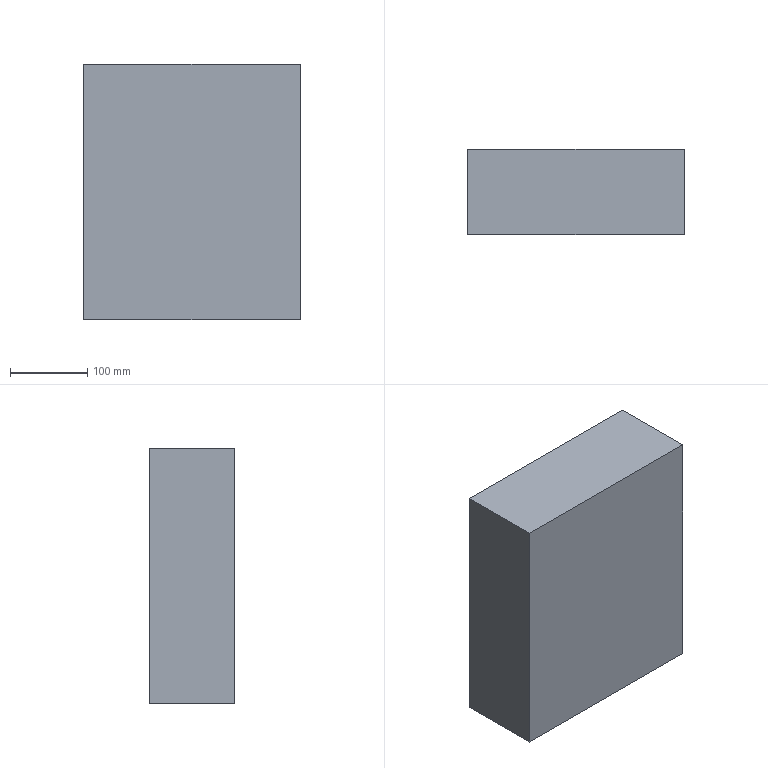Part | STEP file | 0230_Work-A | 1 solid | 6 faces | box 280 x 110 x 330 mm | volume 10164000 mm3 | plane 6
STEP:
#1=CARTESIAN_POINT('',(0.,0.,0.));
#2=DIRECTION('',(0.,0.,1.));
#3=DIRECTION('',(1.,0.,0.));
#4=AXIS2_PLACEMENT_3D('',#1,#2,#3);
#5=CARTESIAN_POINT('',(-140.,0.,-330.));
#6=VERTEX_POINT('',#5);
#7=CARTESIAN_POINT('',(-140.,0.,0.));
#8=VERTEX_POINT('',#7);
#9=CARTESIAN_POINT('',(-140.,0.,0.));
#10=DIRECTION('',(0.,0.,1.));
#11=VECTOR('',#10,1.);
#12=LINE('',#9,#11);
#13=CARTESIAN_POINT('',(-140.,110.,0.));
#14=DIRECTION('',(1.,0.,0.));
#15=DIRECTION('',(0.,0.,-1.));
#16=AXIS2_PLACEMENT_3D('',#13,#14,#15);
#17=PLANE('',#16);
#18=CARTESIAN_POINT('',(0.,-110.));
#19=DIRECTION('',(-1.,0.));
#20=VECTOR('',#19,1.);
#21=LINE('',#18,#20);
#22=(GEOMETRIC_REPRESENTATION_CONTEXT(2)PARAMETRIC_REPRESENTATION_CONTEXT()REPRESENTATION_CONTEXT('',''));
#23=DEFINITIONAL_REPRESENTATION('',(#21),#22);
#24=PCURVE('',#17,#23);
#25=CARTESIAN_POINT('',(-140.,0.,-330.));
#26=DIRECTION('',(0.,-1.,0.));
#27=DIRECTION('',(0.,0.,-1.));
#28=AXIS2_PLACEMENT_3D('',#25,#26,#27);
#29=PLANE('',#28);
#30=CARTESIAN_POINT('',(-330.,0.));
#31=DIRECTION('',(-1.,0.));
#32=VECTOR('',#31,1.);
#33=LINE('',#30,#32);
#34=(GEOMETRIC_REPRESENTATION_CONTEXT(2)PARAMETRIC_REPRESENTATION_CONTEXT()REPRESENTATION_CONTEXT('',''));
#35=DEFINITIONAL_REPRESENTATION('',(#33),#34);
#36=PCURVE('',#29,#35);
#37=SURFACE_CURVE('',#12,(#24,#36),.PCURVE_S1.);
#38=EDGE_CURVE('',#6,#8,#37,.T.);
#39=ORIENTED_EDGE('',*,*,#38,.T.);
#40=CARTESIAN_POINT('',(-140.,110.,0.));
#41=VERTEX_POINT('',#40);
#42=CARTESIAN_POINT('',(-140.,110.,0.));
#43=DIRECTION('',(0.,-1.,0.));
#44=VECTOR('',#43,1.);
#45=LINE('',#42,#44);
#46=CARTESIAN_POINT('',(0.,0.));
#47=DIRECTION('',(0.,-1.));
#48=VECTOR('',#47,1.);
#49=LINE('',#46,#48);
#50=(GEOMETRIC_REPRESENTATION_CONTEXT(2)PARAMETRIC_REPRESENTATION_CONTEXT()REPRESENTATION_CONTEXT('',''));
#51=DEFINITIONAL_REPRESENTATION('',(#49),#50);
#52=PCURVE('',#17,#51);
#53=CARTESIAN_POINT('',(-140.,110.,0.));
#54=DIRECTION('',(0.,0.,-1.));
#55=DIRECTION('',(-1.,0.,0.));
#56=AXIS2_PLACEMENT_3D('',#53,#54,#55);
#57=PLANE('',#56);
#58=CARTESIAN_POINT('',(0.,0.));
#59=DIRECTION('',(0.,-1.));
#60=VECTOR('',#59,1.);
#61=LINE('',#58,#60);
#62=(GEOMETRIC_REPRESENTATION_CONTEXT(2)PARAMETRIC_REPRESENTATION_CONTEXT()REPRESENTATION_CONTEXT('',''));
#63=DEFINITIONAL_REPRESENTATION('',(#61),#62);
#64=PCURVE('',#57,#63);
#65=SURFACE_CURVE('',#45,(#52,#64),.PCURVE_S1.);
#66=EDGE_CURVE('',#41,#8,#65,.T.);
#67=ORIENTED_EDGE('',*,*,#66,.F.);
#68=CARTESIAN_POINT('',(-140.,110.,-330.));
#69=VERTEX_POINT('',#68);
#70=CARTESIAN_POINT('',(-140.,110.,0.));
#71=DIRECTION('',(0.,0.,1.));
#72=VECTOR('',#71,1.);
#73=LINE('',#70,#72);
#74=CARTESIAN_POINT('',(0.,0.));
#75=DIRECTION('',(-1.,0.));
#76=VECTOR('',#75,1.);
#77=LINE('',#74,#76);
#78=(GEOMETRIC_REPRESENTATION_CONTEXT(2)PARAMETRIC_REPRESENTATION_CONTEXT()REPRESENTATION_CONTEXT('',''));
#79=DEFINITIONAL_REPRESENTATION('',(#77),#78);
#80=PCURVE('',#17,#79);
#81=CARTESIAN_POINT('',(-140.,110.,-330.));
#82=DIRECTION('',(0.,-1.,0.));
#83=DIRECTION('',(0.,0.,-1.));
#84=AXIS2_PLACEMENT_3D('',#81,#82,#83);
#85=PLANE('',#84);
#86=CARTESIAN_POINT('',(-330.,0.));
#87=DIRECTION('',(-1.,0.));
#88=VECTOR('',#87,1.);
#89=LINE('',#86,#88);
#90=(GEOMETRIC_REPRESENTATION_CONTEXT(2)PARAMETRIC_REPRESENTATION_CONTEXT()REPRESENTATION_CONTEXT('',''));
#91=DEFINITIONAL_REPRESENTATION('',(#89),#90);
#92=PCURVE('',#85,#91);
#93=SURFACE_CURVE('',#73,(#80,#92),.PCURVE_S1.);
#94=EDGE_CURVE('',#69,#41,#93,.T.);
#95=ORIENTED_EDGE('',*,*,#94,.F.);
#96=CARTESIAN_POINT('',(-140.,110.,-330.));
#97=DIRECTION('',(0.,-1.,0.));
#98=VECTOR('',#97,1.);
#99=LINE('',#96,#98);
#100=CARTESIAN_POINT('',(330.,0.));
#101=DIRECTION('',(0.,-1.));
#102=VECTOR('',#101,1.);
#103=LINE('',#100,#102);
#104=(GEOMETRIC_REPRESENTATION_CONTEXT(2)PARAMETRIC_REPRESENTATION_CONTEXT()REPRESENTATION_CONTEXT('',''));
#105=DEFINITIONAL_REPRESENTATION('',(#103),#104);
#106=PCURVE('',#17,#105);
#107=CARTESIAN_POINT('',(-140.,110.,-330.));
#108=DIRECTION('',(0.,0.,1.));
#109=DIRECTION('',(1.,0.,0.));
#110=AXIS2_PLACEMENT_3D('',#107,#108,#109);
#111=PLANE('',#110);
#112=CARTESIAN_POINT('',(0.,0.));
#113=DIRECTION('',(0.,-1.));
#114=VECTOR('',#113,1.);
#115=LINE('',#112,#114);
#116=(GEOMETRIC_REPRESENTATION_CONTEXT(2)PARAMETRIC_REPRESENTATION_CONTEXT()REPRESENTATION_CONTEXT('',''));
#117=DEFINITIONAL_REPRESENTATION('',(#115),#116);
#118=PCURVE('',#111,#117);
#119=SURFACE_CURVE('',#99,(#106,#118),.PCURVE_S1.);
#120=EDGE_CURVE('',#69,#6,#119,.T.);
#121=ORIENTED_EDGE('',*,*,#120,.T.);
#122=EDGE_LOOP('',(#39,#67,#95,#121));
#123=FACE_BOUND('',#122,.T.);
#124=ADVANCED_FACE('',(#123),#17,.F.);
#125=CARTESIAN_POINT('',(140.,0.,0.));
#126=VERTEX_POINT('',#125);
#127=CARTESIAN_POINT('',(-140.,0.,0.));
#128=DIRECTION('',(1.,0.,0.));
#129=VECTOR('',#128,1.);
#130=LINE('',#127,#129);
#131=CARTESIAN_POINT('',(0.,-110.));
#132=DIRECTION('',(-1.,0.));
#133=VECTOR('',#132,1.);
#134=LINE('',#131,#133);
#135=(GEOMETRIC_REPRESENTATION_CONTEXT(2)PARAMETRIC_REPRESENTATION_CONTEXT()REPRESENTATION_CONTEXT('',''));
#136=DEFINITIONAL_REPRESENTATION('',(#134),#135);
#137=PCURVE('',#57,#136);
#138=CARTESIAN_POINT('',(-330.,0.));
#139=DIRECTION('',(0.,1.));
#140=VECTOR('',#139,1.);
#141=LINE('',#138,#140);
#142=(GEOMETRIC_REPRESENTATION_CONTEXT(2)PARAMETRIC_REPRESENTATION_CONTEXT()REPRESENTATION_CONTEXT('',''));
#143=DEFINITIONAL_REPRESENTATION('',(#141),#142);
#144=PCURVE('',#29,#143);
#145=SURFACE_CURVE('',#130,(#137,#144),.PCURVE_S1.);
#146=EDGE_CURVE('',#8,#126,#145,.T.);
#147=ORIENTED_EDGE('',*,*,#146,.T.);
#148=CARTESIAN_POINT('',(140.,110.,0.));
#149=VERTEX_POINT('',#148);
#150=CARTESIAN_POINT('',(140.,110.,0.));
#151=DIRECTION('',(0.,-1.,0.));
#152=VECTOR('',#151,1.);
#153=LINE('',#150,#152);
#154=CARTESIAN_POINT('',(-280.,0.));
#155=DIRECTION('',(0.,-1.));
#156=VECTOR('',#155,1.);
#157=LINE('',#154,#156);
#158=(GEOMETRIC_REPRESENTATION_CONTEXT(2)PARAMETRIC_REPRESENTATION_CONTEXT()REPRESENTATION_CONTEXT('',''));
#159=DEFINITIONAL_REPRESENTATION('',(#157),#158);
#160=PCURVE('',#57,#159);
#161=CARTESIAN_POINT('',(140.,110.,0.));
#162=DIRECTION('',(-1.,0.,0.));
#163=DIRECTION('',(0.,0.,1.));
#164=AXIS2_PLACEMENT_3D('',#161,#162,#163);
#165=PLANE('',#164);
#166=CARTESIAN_POINT('',(0.,0.));
#167=DIRECTION('',(0.,-1.));
#168=VECTOR('',#167,1.);
#169=LINE('',#166,#168);
#170=(GEOMETRIC_REPRESENTATION_CONTEXT(2)PARAMETRIC_REPRESENTATION_CONTEXT()REPRESENTATION_CONTEXT('',''));
#171=DEFINITIONAL_REPRESENTATION('',(#169),#170);
#172=PCURVE('',#165,#171);
#173=SURFACE_CURVE('',#153,(#160,#172),.PCURVE_S1.);
#174=EDGE_CURVE('',#149,#126,#173,.T.);
#175=ORIENTED_EDGE('',*,*,#174,.F.);
#176=CARTESIAN_POINT('',(-140.,110.,0.));
#177=DIRECTION('',(1.,0.,0.));
#178=VECTOR('',#177,1.);
#179=LINE('',#176,#178);
#180=CARTESIAN_POINT('',(0.,0.));
#181=DIRECTION('',(-1.,0.));
#182=VECTOR('',#181,1.);
#183=LINE('',#180,#182);
#184=(GEOMETRIC_REPRESENTATION_CONTEXT(2)PARAMETRIC_REPRESENTATION_CONTEXT()REPRESENTATION_CONTEXT('',''));
#185=DEFINITIONAL_REPRESENTATION('',(#183),#184);
#186=PCURVE('',#57,#185);
#187=CARTESIAN_POINT('',(-330.,0.));
#188=DIRECTION('',(0.,1.));
#189=VECTOR('',#188,1.);
#190=LINE('',#187,#189);
#191=(GEOMETRIC_REPRESENTATION_CONTEXT(2)PARAMETRIC_REPRESENTATION_CONTEXT()REPRESENTATION_CONTEXT('',''));
#192=DEFINITIONAL_REPRESENTATION('',(#190),#191);
#193=PCURVE('',#85,#192);
#194=SURFACE_CURVE('',#179,(#186,#193),.PCURVE_S1.);
#195=EDGE_CURVE('',#41,#149,#194,.T.);
#196=ORIENTED_EDGE('',*,*,#195,.F.);
#197=ORIENTED_EDGE('',*,*,#66,.T.);
#198=EDGE_LOOP('',(#147,#175,#196,#197));
#199=FACE_BOUND('',#198,.T.);
#200=ADVANCED_FACE('',(#199),#57,.F.);
#201=CARTESIAN_POINT('',(140.,0.,-330.));
#202=VERTEX_POINT('',#201);
#203=CARTESIAN_POINT('',(140.,0.,0.));
#204=DIRECTION('',(0.,0.,-1.));
#205=VECTOR('',#204,1.);
#206=LINE('',#203,#205);
#207=CARTESIAN_POINT('',(0.,-110.));
#208=DIRECTION('',(-1.,0.));
#209=VECTOR('',#208,1.);
#210=LINE('',#207,#209);
#211=(GEOMETRIC_REPRESENTATION_CONTEXT(2)PARAMETRIC_REPRESENTATION_CONTEXT()REPRESENTATION_CONTEXT('',''));
#212=DEFINITIONAL_REPRESENTATION('',(#210),#211);
#213=PCURVE('',#165,#212);
#214=CARTESIAN_POINT('',(-330.,280.));
#215=DIRECTION('',(1.,0.));
#216=VECTOR('',#215,1.);
#217=LINE('',#214,#216);
#218=(GEOMETRIC_REPRESENTATION_CONTEXT(2)PARAMETRIC_REPRESENTATION_CONTEXT()REPRESENTATION_CONTEXT('',''));
#219=DEFINITIONAL_REPRESENTATION('',(#217),#218);
#220=PCURVE('',#29,#219);
#221=SURFACE_CURVE('',#206,(#213,#220),.PCURVE_S1.);
#222=EDGE_CURVE('',#126,#202,#221,.T.);
#223=ORIENTED_EDGE('',*,*,#222,.T.);
#224=CARTESIAN_POINT('',(140.,110.,-330.));
#225=VERTEX_POINT('',#224);
#226=CARTESIAN_POINT('',(140.,110.,-330.));
#227=DIRECTION('',(0.,-1.,0.));
#228=VECTOR('',#227,1.);
#229=LINE('',#226,#228);
#230=CARTESIAN_POINT('',(-330.,0.));
#231=DIRECTION('',(0.,-1.));
#232=VECTOR('',#231,1.);
#233=LINE('',#230,#232);
#234=(GEOMETRIC_REPRESENTATION_CONTEXT(2)PARAMETRIC_REPRESENTATION_CONTEXT()REPRESENTATION_CONTEXT('',''));
#235=DEFINITIONAL_REPRESENTATION('',(#233),#234);
#236=PCURVE('',#165,#235);
#237=CARTESIAN_POINT('',(280.,0.));
#238=DIRECTION('',(0.,-1.));
#239=VECTOR('',#238,1.);
#240=LINE('',#237,#239);
#241=(GEOMETRIC_REPRESENTATION_CONTEXT(2)PARAMETRIC_REPRESENTATION_CONTEXT()REPRESENTATION_CONTEXT('',''));
#242=DEFINITIONAL_REPRESENTATION('',(#240),#241);
#243=PCURVE('',#111,#242);
#244=SURFACE_CURVE('',#229,(#236,#243),.PCURVE_S1.);
#245=EDGE_CURVE('',#225,#202,#244,.T.);
#246=ORIENTED_EDGE('',*,*,#245,.F.);
#247=CARTESIAN_POINT('',(140.,110.,0.));
#248=DIRECTION('',(0.,0.,-1.));
#249=VECTOR('',#248,1.);
#250=LINE('',#247,#249);
#251=CARTESIAN_POINT('',(0.,0.));
#252=DIRECTION('',(-1.,0.));
#253=VECTOR('',#252,1.);
#254=LINE('',#251,#253);
#255=(GEOMETRIC_REPRESENTATION_CONTEXT(2)PARAMETRIC_REPRESENTATION_CONTEXT()REPRESENTATION_CONTEXT('',''));
#256=DEFINITIONAL_REPRESENTATION('',(#254),#255);
#257=PCURVE('',#165,#256);
#258=CARTESIAN_POINT('',(-330.,280.));
#259=DIRECTION('',(1.,0.));
#260=VECTOR('',#259,1.);
#261=LINE('',#258,#260);
#262=(GEOMETRIC_REPRESENTATION_CONTEXT(2)PARAMETRIC_REPRESENTATION_CONTEXT()REPRESENTATION_CONTEXT('',''));
#263=DEFINITIONAL_REPRESENTATION('',(#261),#262);
#264=PCURVE('',#85,#263);
#265=SURFACE_CURVE('',#250,(#257,#264),.PCURVE_S1.);
#266=EDGE_CURVE('',#149,#225,#265,.T.);
#267=ORIENTED_EDGE('',*,*,#266,.F.);
#268=ORIENTED_EDGE('',*,*,#174,.T.);
#269=EDGE_LOOP('',(#223,#246,#267,#268));
#270=FACE_BOUND('',#269,.T.);
#271=ADVANCED_FACE('',(#270),#165,.F.);
#272=CARTESIAN_POINT('',(-140.,0.,-330.));
#273=DIRECTION('',(-1.,0.,0.));
#274=VECTOR('',#273,1.);
#275=LINE('',#272,#274);
#276=CARTESIAN_POINT('',(0.,-110.));
#277=DIRECTION('',(-1.,0.));
#278=VECTOR('',#277,1.);
#279=LINE('',#276,#278);
#280=(GEOMETRIC_REPRESENTATION_CONTEXT(2)PARAMETRIC_REPRESENTATION_CONTEXT()REPRESENTATION_CONTEXT('',''));
#281=DEFINITIONAL_REPRESENTATION('',(#279),#280);
#282=PCURVE('',#111,#281);
#283=CARTESIAN_POINT('',(0.,0.));
#284=DIRECTION('',(0.,-1.));
#285=VECTOR('',#284,1.);
#286=LINE('',#283,#285);
#287=(GEOMETRIC_REPRESENTATION_CONTEXT(2)PARAMETRIC_REPRESENTATION_CONTEXT()REPRESENTATION_CONTEXT('',''));
#288=DEFINITIONAL_REPRESENTATION('',(#286),#287);
#289=PCURVE('',#29,#288);
#290=SURFACE_CURVE('',#275,(#282,#289),.PCURVE_S1.);
#291=EDGE_CURVE('',#202,#6,#290,.T.);
#292=ORIENTED_EDGE('',*,*,#291,.T.);
#293=ORIENTED_EDGE('',*,*,#120,.F.);
#294=CARTESIAN_POINT('',(-140.,110.,-330.));
#295=DIRECTION('',(-1.,0.,0.));
#296=VECTOR('',#295,1.);
#297=LINE('',#294,#296);
#298=CARTESIAN_POINT('',(0.,0.));
#299=DIRECTION('',(-1.,0.));
#300=VECTOR('',#299,1.);
#301=LINE('',#298,#300);
#302=(GEOMETRIC_REPRESENTATION_CONTEXT(2)PARAMETRIC_REPRESENTATION_CONTEXT()REPRESENTATION_CONTEXT('',''));
#303=DEFINITIONAL_REPRESENTATION('',(#301),#302);
#304=PCURVE('',#111,#303);
#305=CARTESIAN_POINT('',(0.,0.));
#306=DIRECTION('',(0.,-1.));
#307=VECTOR('',#306,1.);
#308=LINE('',#305,#307);
#309=(GEOMETRIC_REPRESENTATION_CONTEXT(2)PARAMETRIC_REPRESENTATION_CONTEXT()REPRESENTATION_CONTEXT('',''));
#310=DEFINITIONAL_REPRESENTATION('',(#308),#309);
#311=PCURVE('',#85,#310);
#312=SURFACE_CURVE('',#297,(#304,#311),.PCURVE_S1.);
#313=EDGE_CURVE('',#225,#69,#312,.T.);
#314=ORIENTED_EDGE('',*,*,#313,.F.);
#315=ORIENTED_EDGE('',*,*,#245,.T.);
#316=EDGE_LOOP('',(#292,#293,#314,#315));
#317=FACE_BOUND('',#316,.T.);
#318=ADVANCED_FACE('',(#317),#111,.F.);
#319=ORIENTED_EDGE('',*,*,#94,.T.);
#320=ORIENTED_EDGE('',*,*,#195,.T.);
#321=ORIENTED_EDGE('',*,*,#266,.T.);
#322=ORIENTED_EDGE('',*,*,#313,.T.);
#323=EDGE_LOOP('',(#319,#320,#321,#322));
#324=FACE_BOUND('',#323,.T.);
#325=ADVANCED_FACE('',(#324),#85,.F.);
#326=ORIENTED_EDGE('',*,*,#38,.F.);
#327=ORIENTED_EDGE('',*,*,#291,.F.);
#328=ORIENTED_EDGE('',*,*,#222,.F.);
#329=ORIENTED_EDGE('',*,*,#146,.F.);
#330=EDGE_LOOP('',(#326,#327,#328,#329));
#331=FACE_BOUND('',#330,.T.);
#332=ADVANCED_FACE('',(#331),#29,.T.);
#333=CLOSED_SHELL('',(#124,#200,#271,#318,#325,#332));
#334=MANIFOLD_SOLID_BREP('',#333);
#335=(LENGTH_UNIT()NAMED_UNIT(*)SI_UNIT(.MILLI.,.METRE.));
#336=UNCERTAINTY_MEASURE_WITH_UNIT(LENGTH_MEASURE(0.0000001),#335,'','');
#337=(NAMED_UNIT(*)PLANE_ANGLE_UNIT()SI_UNIT($,.RADIAN.));
#338=(NAMED_UNIT(*)SI_UNIT($,.STERADIAN.)SOLID_ANGLE_UNIT());
#339=(GEOMETRIC_REPRESENTATION_CONTEXT(3)GLOBAL_UNCERTAINTY_ASSIGNED_CONTEXT((#336))GLOBAL_UNIT_ASSIGNED_CONTEXT((#335,#337,#338))REPRESENTATION_CONTEXT('',''));
#340=ADVANCED_BREP_SHAPE_REPRESENTATION('',(#4,#334),#339);